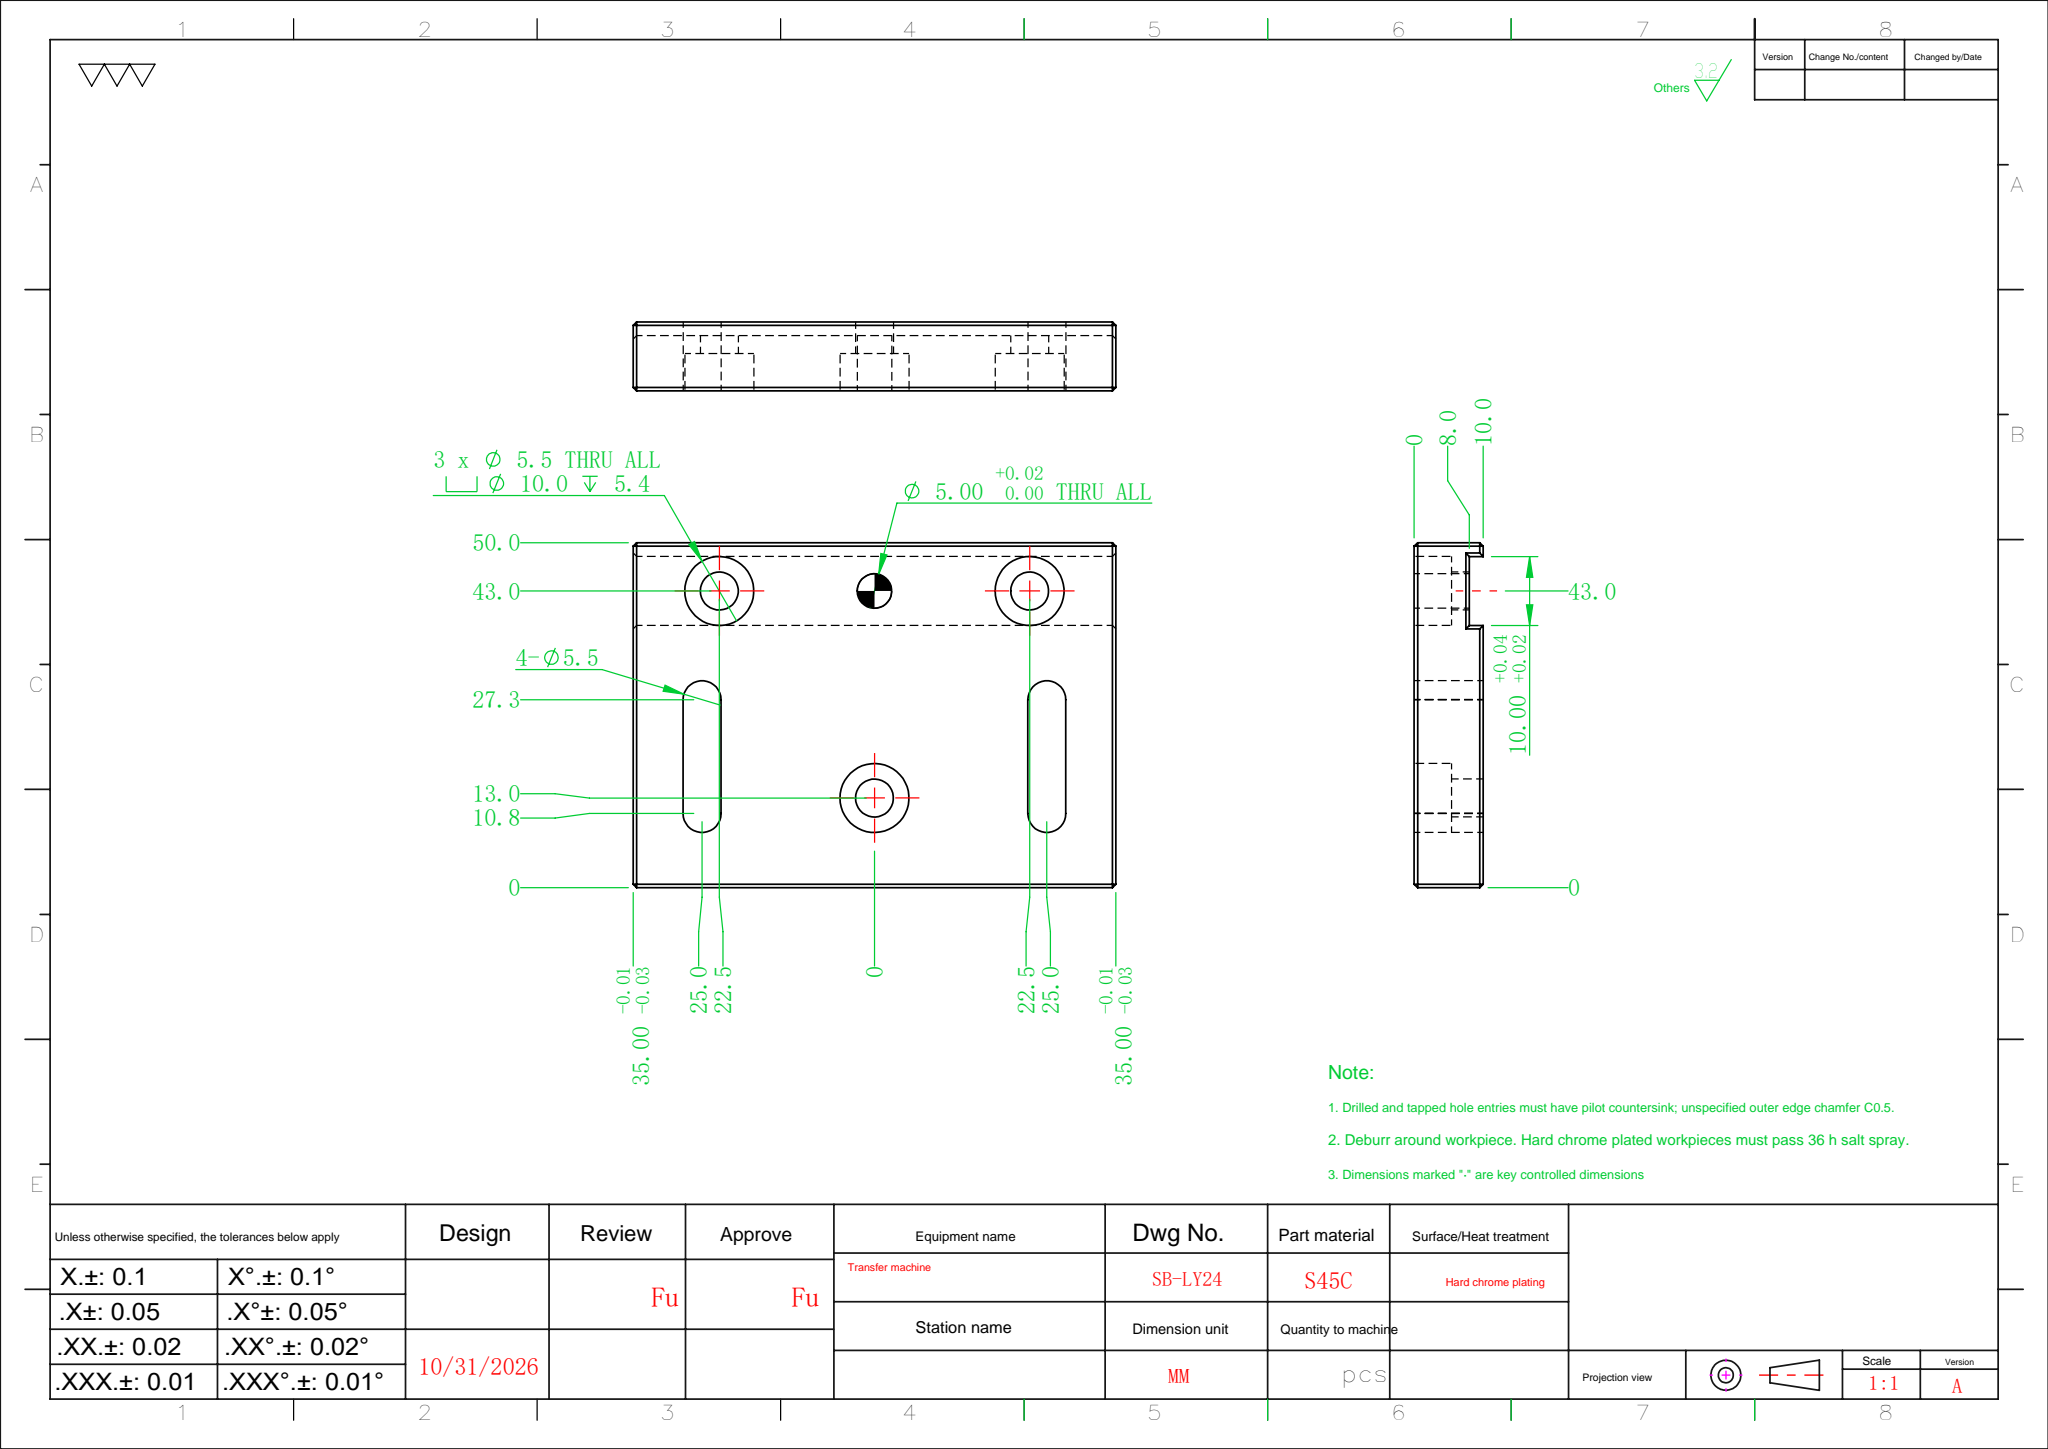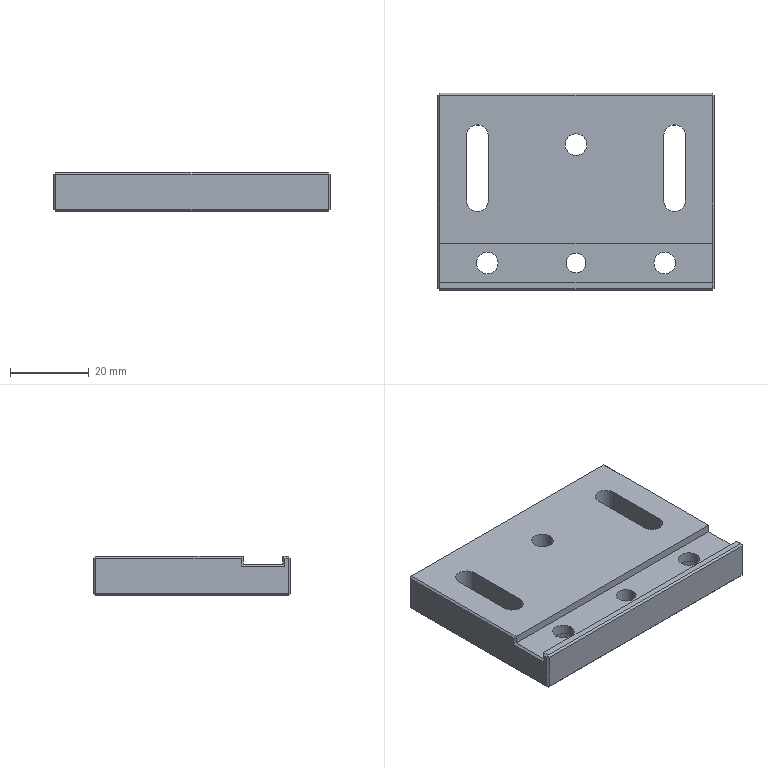Part | SolidWorks | features HoleWzd 3, Chamfer 1, Cut 1, Extrusion 1 | 1 solid | 63 faces | box 70 x 50 x 10 mm | volume 29582 mm3 | plane 45 | cylinder 18 | commonest cylinder face diameters 5.5 x10 10 x6 5 x2